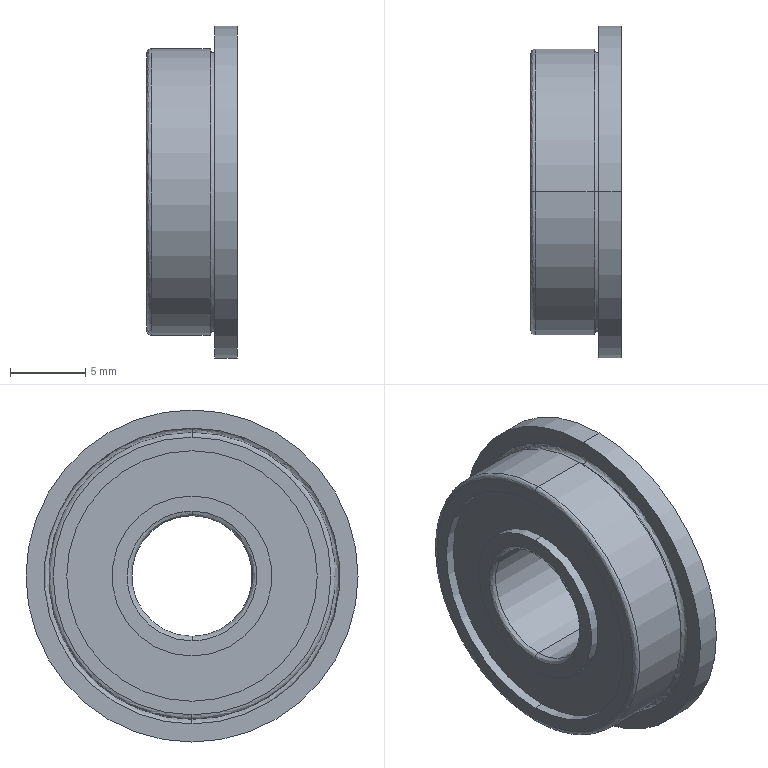Part | SolidWorks | features BaseBody 1 | 1 solid | 31 faces | box 6 x 22 x 22 mm | volume 1366 mm3 | cylinder 14 | spline 11 | plane 6 | commonest cylinder face diameters 10.6 x4 16.6 x4 8 x2 19 x2 22 x2
STEP:
#1=CARTESIAN_POINT('',(4.5,0.,-9.2));
#2=VERTEX_POINT('',#1);
#3=CARTESIAN_POINT('',(4.5,0.,9.2));
#4=VERTEX_POINT('',#3);
#5=CARTESIAN_POINT('',(4.5,0.,0.));
#6=DIRECTION('',(-1.,0.,0.));
#7=DIRECTION('',(0.,0.,1.));
#8=AXIS2_PLACEMENT_3D('',#5,#6,#7);
#9=CIRCLE('',#8,9.2);
#10=EDGE_CURVE('',#2,#4,#9,.T.);
#11=ORIENTED_EDGE('',*,*,#10,.F.);
#12=CARTESIAN_POINT('',(4.5,0.,-9.8));
#13=VERTEX_POINT('',#12);
#14=CARTESIAN_POINT('',(4.5,0.,-9.5));
#15=DIRECTION('',(0.,1.,0.));
#16=DIRECTION('',(0.,0.,1.));
#17=AXIS2_PLACEMENT_3D('',#14,#15,#16);
#18=CIRCLE('',#17,0.3);
#19=EDGE_CURVE('',#2,#13,#18,.T.);
#20=ORIENTED_EDGE('',*,*,#19,.T.);
#21=CARTESIAN_POINT('',(4.5,0.,9.8));
#22=VERTEX_POINT('',#21);
#23=CARTESIAN_POINT('',(4.5,0.,0.));
#24=DIRECTION('',(-1.,0.,0.));
#25=DIRECTION('',(0.,0.,1.));
#26=AXIS2_PLACEMENT_3D('',#23,#24,#25);
#27=CIRCLE('',#26,9.8);
#28=EDGE_CURVE('',#13,#22,#27,.T.);
#29=ORIENTED_EDGE('',*,*,#28,.T.);
#30=CARTESIAN_POINT('',(4.5,0.,9.5));
#31=DIRECTION('',(0.,-1.,0.));
#32=DIRECTION('',(0.,0.,-1.));
#33=AXIS2_PLACEMENT_3D('',#30,#31,#32);
#34=CIRCLE('',#33,0.3);
#35=EDGE_CURVE('',#4,#22,#34,.T.);
#36=ORIENTED_EDGE('',*,*,#35,.F.);
#37=EDGE_LOOP('',(#11,#20,#29,#36));
#38=FACE_OUTER_BOUND('',#37,.T.);
#39=CARTESIAN_POINT('',(4.5,0.,-9.2));
#40=CARTESIAN_POINT('',(4.5,-18.4,-9.2));
#41=CARTESIAN_POINT('',(4.5,-18.4,9.2));
#42=CARTESIAN_POINT('',(4.5,0.,9.2));
#43=CARTESIAN_POINT('',(5.1,0.,-9.2));
#44=CARTESIAN_POINT('',(5.1,-18.4,-9.2));
#45=CARTESIAN_POINT('',(5.1,-18.4,9.2));
#46=CARTESIAN_POINT('',(5.1,0.,9.2));
#47=CARTESIAN_POINT('',(5.1,0.,-9.8));
#48=CARTESIAN_POINT('',(5.1,-19.6,-9.8));
#49=CARTESIAN_POINT('',(5.1,-19.6,9.8));
#50=CARTESIAN_POINT('',(5.1,0.,9.8));
#51=CARTESIAN_POINT('',(4.5,0.,-9.8));
#52=CARTESIAN_POINT('',(4.5,-19.6,-9.8));
#53=CARTESIAN_POINT('',(4.5,-19.6,9.8));
#54=CARTESIAN_POINT('',(4.5,0.,9.8));
#55=(BOUNDED_SURFACE()B_SPLINE_SURFACE(3,3,((#39,#40,#41,#42),(#43,#44,#45,#46),(#47,#48,#49,#50),(#51,#52,#53,#54)),.UNSPECIFIED.,.F.,.F.,.T.)B_SPLINE_SURFACE_WITH_KNOTS((4,4),(4,4),(0.,1.),(0.,1.),.UNSPECIFIED.)GEOMETRIC_REPRESENTATION_ITEM()RATIONAL_B_SPLINE_SURFACE(((1.,0.3333,0.3333,1.),(0.3333,0.1111,0.1111,0.3333),(0.3333,0.1111,0.1111,0.3333),(1.,0.3333,0.3333,1.)))REPRESENTATION_ITEM('')SURFACE());
#56=ADVANCED_FACE('',(#38),#55,.T.);
#57=CARTESIAN_POINT('',(0.,0.,9.2));
#58=VERTEX_POINT('',#57);
#59=CARTESIAN_POINT('',(0.,0.,-9.2));
#60=VERTEX_POINT('',#59);
#61=CARTESIAN_POINT('',(0.,0.,0.));
#62=DIRECTION('',(1.,0.,0.));
#63=DIRECTION('',(0.,0.,1.));
#64=AXIS2_PLACEMENT_3D('',#61,#62,#63);
#65=CIRCLE('',#64,9.2);
#66=EDGE_CURVE('',#58,#60,#65,.T.);
#67=ORIENTED_EDGE('',*,*,#66,.T.);
#68=CARTESIAN_POINT('',(0.3,0.,-9.5));
#69=VERTEX_POINT('',#68);
#70=CARTESIAN_POINT('',(0.3,0.,-9.2));
#71=DIRECTION('',(0.,-1.,0.));
#72=DIRECTION('',(0.,0.,1.));
#73=AXIS2_PLACEMENT_3D('',#70,#71,#72);
#74=CIRCLE('',#73,0.3);
#75=EDGE_CURVE('',#60,#69,#74,.T.);
#76=ORIENTED_EDGE('',*,*,#75,.T.);
#77=CARTESIAN_POINT('',(0.3,0.,9.5));
#78=VERTEX_POINT('',#77);
#79=CARTESIAN_POINT('',(0.3,0.,0.));
#80=DIRECTION('',(1.,0.,0.));
#81=DIRECTION('',(0.,1.,0.));
#82=AXIS2_PLACEMENT_3D('',#79,#80,#81);
#83=CIRCLE('',#82,9.5);
#84=EDGE_CURVE('',#78,#69,#83,.T.);
#85=ORIENTED_EDGE('',*,*,#84,.F.);
#86=CARTESIAN_POINT('',(0.3,0.,9.2));
#87=DIRECTION('',(0.,1.,0.));
#88=DIRECTION('',(0.,0.,-1.));
#89=AXIS2_PLACEMENT_3D('',#86,#87,#88);
#90=CIRCLE('',#89,0.3);
#91=EDGE_CURVE('',#58,#78,#90,.T.);
#92=ORIENTED_EDGE('',*,*,#91,.F.);
#93=EDGE_LOOP('',(#67,#76,#85,#92));
#94=FACE_OUTER_BOUND('',#93,.T.);
#95=CARTESIAN_POINT('',(0.,0.,-9.2));
#96=CARTESIAN_POINT('',(0.,-18.4,-9.2));
#97=CARTESIAN_POINT('',(0.,-18.4,9.2));
#98=CARTESIAN_POINT('',(0.,0.,9.2));
#99=CARTESIAN_POINT('',(0.,0.,-9.376));
#100=CARTESIAN_POINT('',(0.,-18.751,-9.376));
#101=CARTESIAN_POINT('',(0.,-18.751,9.376));
#102=CARTESIAN_POINT('',(0.,0.,9.376));
#103=CARTESIAN_POINT('',(0.1243,0.,-9.5));
#104=CARTESIAN_POINT('',(0.1243,-19.,-9.5));
#105=CARTESIAN_POINT('',(0.1243,-19.,9.5));
#106=CARTESIAN_POINT('',(0.1243,0.,9.5));
#107=CARTESIAN_POINT('',(0.3,0.,-9.5));
#108=CARTESIAN_POINT('',(0.3,-19.,-9.5));
#109=CARTESIAN_POINT('',(0.3,-19.,9.5));
#110=CARTESIAN_POINT('',(0.3,0.,9.5));
#111=(BOUNDED_SURFACE()B_SPLINE_SURFACE(3,3,((#95,#96,#97,#98),(#99,#100,#101,#102),(#103,#104,#105,#106),(#107,#108,#109,#110)),.UNSPECIFIED.,.F.,.F.,.F.)B_SPLINE_SURFACE_WITH_KNOTS((4,4),(4,4),(0.,1.),(0.,1.),.UNSPECIFIED.)GEOMETRIC_REPRESENTATION_ITEM()RATIONAL_B_SPLINE_SURFACE(((1.,0.3333,0.3333,1.),(0.8047,0.2682,0.2682,0.8047),(0.8047,0.2682,0.2682,0.8047),(1.,0.3333,0.3333,1.)))REPRESENTATION_ITEM('')SURFACE());
#112=ADVANCED_FACE('',(#94),#111,.T.);
#113=CARTESIAN_POINT('',(0.3,0.,4.));
#114=VERTEX_POINT('',#113);
#115=CARTESIAN_POINT('',(0.3,0.,-4.));
#116=VERTEX_POINT('',#115);
#117=CARTESIAN_POINT('',(0.3,0.,0.));
#118=DIRECTION('',(1.,0.,0.));
#119=DIRECTION('',(0.,0.,1.));
#120=AXIS2_PLACEMENT_3D('',#117,#118,#119);
#121=CIRCLE('',#120,4.);
#122=EDGE_CURVE('',#114,#116,#121,.T.);
#123=ORIENTED_EDGE('',*,*,#122,.T.);
#124=CARTESIAN_POINT('',(0.,0.,-4.3));
#125=VERTEX_POINT('',#124);
#126=CARTESIAN_POINT('',(0.3,0.,-4.3));
#127=DIRECTION('',(0.,-1.,0.));
#128=DIRECTION('',(0.,0.,1.));
#129=AXIS2_PLACEMENT_3D('',#126,#127,#128);
#130=CIRCLE('',#129,0.3);
#131=EDGE_CURVE('',#116,#125,#130,.T.);
#132=ORIENTED_EDGE('',*,*,#131,.T.);
#133=CARTESIAN_POINT('',(0.,0.,4.3));
#134=VERTEX_POINT('',#133);
#135=CARTESIAN_POINT('',(0.,0.,4.3));
#136=CARTESIAN_POINT('',(0.,-0.2048,4.3));
#137=CARTESIAN_POINT('',(0.,-0.509,4.278));
#138=CARTESIAN_POINT('',(0.,-0.8583,4.216));
#139=CARTESIAN_POINT('',(0.,-1.032,4.175));
#140=CARTESIAN_POINT('',(0.,-1.118,4.152));
#141=CARTESIAN_POINT('',(0.,-1.161,4.14));
#142=CARTESIAN_POINT('',(0.,-1.179,4.135));
#143=CARTESIAN_POINT('',(0.,-1.192,4.132));
#144=CARTESIAN_POINT('',(0.,-1.196,4.13));
#145=CARTESIAN_POINT('',(0.,-1.454,4.055));
#146=CARTESIAN_POINT('',(0.,-1.814,3.914));
#147=CARTESIAN_POINT('',(0.,-2.206,3.695));
#148=CARTESIAN_POINT('',(0.,-2.395,3.572));
#149=CARTESIAN_POINT('',(0.,-2.488,3.507));
#150=CARTESIAN_POINT('',(0.,-2.534,3.474));
#151=CARTESIAN_POINT('',(0.,-2.554,3.459));
#152=CARTESIAN_POINT('',(0.,-2.567,3.45));
#153=CARTESIAN_POINT('',(0.,-2.572,3.446));
#154=CARTESIAN_POINT('',(0.,-2.701,3.35));
#155=CARTESIAN_POINT('',(0.,-2.873,3.205));
#156=CARTESIAN_POINT('',(0.,-3.061,3.021));
#157=CARTESIAN_POINT('',(0.,-3.152,2.926));
#158=CARTESIAN_POINT('',(0.,-3.19,2.884));
#159=CARTESIAN_POINT('',(0.,-3.215,2.856));
#160=CARTESIAN_POINT('',(0.,-3.226,2.843));
#161=CARTESIAN_POINT('',(0.,-3.347,2.704));
#162=CARTESIAN_POINT('',(0.,-3.497,2.511));
#163=CARTESIAN_POINT('',(0.,-3.652,2.272));
#164=CARTESIAN_POINT('',(0.,-3.725,2.149));
#165=CARTESIAN_POINT('',(0.,-3.755,2.095));
#166=CARTESIAN_POINT('',(0.,-3.775,2.06));
#167=CARTESIAN_POINT('',(0.,-3.784,2.043));
#168=CARTESIAN_POINT('',(0.,-3.876,1.87));
#169=CARTESIAN_POINT('',(0.,-3.984,1.635));
#170=CARTESIAN_POINT('',(0.,-4.084,1.35));
#171=CARTESIAN_POINT('',(0.,-4.122,1.226));
#172=CARTESIAN_POINT('',(0.,-4.146,1.143));
#173=CARTESIAN_POINT('',(0.,-4.157,1.102));
#174=CARTESIAN_POINT('',(0.,-4.256,0.7117));
#175=CARTESIAN_POINT('',(0.,-4.3,0.3578));
#176=CARTESIAN_POINT('',(0.,-4.3,-0.1789));
#177=CARTESIAN_POINT('',(0.,-4.284,-0.4454));
#178=CARTESIAN_POINT('',(0.,-4.235,-0.753));
#179=CARTESIAN_POINT('',(0.,-4.208,-0.8842));
#180=CARTESIAN_POINT('',(0.,-4.189,-0.9714));
#181=CARTESIAN_POINT('',(0.,-4.178,-1.016));
#182=CARTESIAN_POINT('',(0.,-4.125,-1.227));
#183=CARTESIAN_POINT('',(0.,-4.046,-1.473));
#184=CARTESIAN_POINT('',(0.,-3.929,-1.752));
#185=CARTESIAN_POINT('',(0.,-3.864,-1.888));
#186=CARTESIAN_POINT('',(0.,-3.834,-1.947));
#187=CARTESIAN_POINT('',(0.,-3.814,-1.985));
#188=CARTESIAN_POINT('',(0.,-3.804,-2.005));
#189=CARTESIAN_POINT('',(0.,-3.717,-2.168));
#190=CARTESIAN_POINT('',(0.,-3.59,-2.377));
#191=CARTESIAN_POINT('',(0.,-3.422,-2.607));
#192=CARTESIAN_POINT('',(0.,-3.332,-2.718));
#193=CARTESIAN_POINT('',(0.,-3.293,-2.765));
#194=CARTESIAN_POINT('',(0.,-3.267,-2.796));
#195=CARTESIAN_POINT('',(0.,-3.252,-2.813));
#196=CARTESIAN_POINT('',(0.,-3.141,-2.941));
#197=CARTESIAN_POINT('',(0.,-2.984,-3.103));
#198=CARTESIAN_POINT('',(0.,-2.787,-3.276));
#199=CARTESIAN_POINT('',(0.,-2.685,-3.359));
#200=CARTESIAN_POINT('',(0.,-2.633,-3.4));
#201=CARTESIAN_POINT('',(0.,-2.61,-3.417));
#202=CARTESIAN_POINT('',(0.,-2.595,-3.429));
#203=CARTESIAN_POINT('',(0.,-2.587,-3.435));
#204=CARTESIAN_POINT('',(0.,-2.372,-3.596));
#205=CARTESIAN_POINT('',(0.,-2.043,-3.799));
#206=CARTESIAN_POINT('',(0.,-1.633,-3.982));
#207=CARTESIAN_POINT('',(0.,-1.421,-4.06));
#208=CARTESIAN_POINT('',(0.,-1.313,-4.095));
#209=CARTESIAN_POINT('',(0.,-1.259,-4.112));
#210=CARTESIAN_POINT('',(0.,-1.235,-4.119));
#211=CARTESIAN_POINT('',(0.,-1.22,-4.123));
#212=CARTESIAN_POINT('',(0.,-1.21,-4.126));
#213=CARTESIAN_POINT('',(0.,-0.8114,-4.243));
#214=CARTESIAN_POINT('',(0.,-0.41,-4.3));
#215=CARTESIAN_POINT('',(0.,0.,-4.3));
#216=B_SPLINE_CURVE_WITH_KNOTS('',3,(#135,#136,#137,#138,#139,#140,#141,#142,#143,#144,#145,#146,#147,#148,#149,#150,#151,#152,#153,#154,#155,#156,#157,#158,#159,#160,#161,#162,#163,#164,#165,#166,#167,#168,#169,#170,#171,#172,#173,#174,#175,#176,#177,#178,#179,#180,#181,#182,#183,#184,#185,#186,#187,#188,#189,#190,#191,#192,#193,#194,#195,#196,#197,#198,#199,#200,#201,#202,#203,#204,#205,#206,#207,#208,#209,#210,#211,#212,#213,#214,#215),.UNSPECIFIED.,.F.,.F.,(4,1,1,1,1,1,2,2,1,1,1,1,1,2,2,1,1,1,2,2,1,1,1,2,2,1,1,2,2,2,1,1,2,2,1,1,1,2,2,1,1,1,2,2,1,1,1,1,2,2,1,1,1,1,1,2,2,4),(0.,0.0625,0.09375,0.1094,0.1172,0.1211,0.123,0.125,0.1875,0.2187,0.2344,0.2422,0.2461,0.248,0.25,0.2812,0.2969,0.3047,0.3086,0.3125,0.3437,0.3594,0.3672,0.3711,0.375,0.4062,0.4219,0.4297,0.4375,0.5,0.5312,0.5469,0.5547,0.5625,0.5937,0.6094,0.6172,0.6211,0.625,0.6562,0.6719,0.6797,0.6836,0.6875,0.7187,0.7344,0.7422,0.7461,0.748,0.75,0.8125,0.8437,0.8594,0.8672,0.8711,0.873,0.875,1.),.UNSPECIFIED.);
#217=EDGE_CURVE('',#134,#125,#216,.T.);
#218=ORIENTED_EDGE('',*,*,#217,.F.);
#219=CARTESIAN_POINT('',(0.3,0.,4.3));
#220=DIRECTION('',(0.,1.,0.));
#221=DIRECTION('',(0.,0.,-1.));
#222=AXIS2_PLACEMENT_3D('',#219,#220,#221);
#223=CIRCLE('',#222,0.3);
#224=EDGE_CURVE('',#114,#134,#223,.T.);
#225=ORIENTED_EDGE('',*,*,#224,.F.);
#226=EDGE_LOOP('',(#123,#132,#218,#225));
#227=FACE_OUTER_BOUND('',#226,.T.);
#228=CARTESIAN_POINT('',(0.3,0.,-4.));
#229=CARTESIAN_POINT('',(0.3,-8.,-4.));
#230=CARTESIAN_POINT('',(0.3,-8.,4.));
#231=CARTESIAN_POINT('',(0.3,0.,4.));
#232=CARTESIAN_POINT('',(0.1243,0.,-4.));
#233=CARTESIAN_POINT('',(0.1243,-8.,-4.));
#234=CARTESIAN_POINT('',(0.1243,-8.,4.));
#235=CARTESIAN_POINT('',(0.1243,0.,4.));
#236=CARTESIAN_POINT('',(0.,0.,-4.124));
#237=CARTESIAN_POINT('',(0.,-8.249,-4.124));
#238=CARTESIAN_POINT('',(0.,-8.249,4.124));
#239=CARTESIAN_POINT('',(0.,0.,4.124));
#240=CARTESIAN_POINT('',(0.,0.,-4.3));
#241=CARTESIAN_POINT('',(0.,-8.6,-4.3));
#242=CARTESIAN_POINT('',(0.,-8.6,4.3));
#243=CARTESIAN_POINT('',(0.,0.,4.3));
#244=(BOUNDED_SURFACE()B_SPLINE_SURFACE(3,3,((#228,#229,#230,#231),(#232,#233,#234,#235),(#236,#237,#238,#239),(#240,#241,#242,#243)),.UNSPECIFIED.,.F.,.F.,.T.)B_SPLINE_SURFACE_WITH_KNOTS((4,4),(4,4),(0.,1.),(0.,1.),.UNSPECIFIED.)GEOMETRIC_REPRESENTATION_ITEM()RATIONAL_B_SPLINE_SURFACE(((1.,0.3333,0.3333,1.),(0.8047,0.2682,0.2682,0.8047),(0.8047,0.2682,0.2682,0.8047),(1.,0.3333,0.3333,1.)))REPRESENTATION_ITEM('')SURFACE());
#245=ADVANCED_FACE('',(#227),#244,.T.);
#246=CARTESIAN_POINT('',(6.,0.,-4.3));
#247=VERTEX_POINT('',#246);
#248=CARTESIAN_POINT('',(6.,0.,4.3));
#249=VERTEX_POINT('',#248);
#250=CARTESIAN_POINT('',(6.,0.,-4.3));
#251=CARTESIAN_POINT('',(6.,-0.2048,-4.3));
#252=CARTESIAN_POINT('',(6.,-0.509,-4.278));
#253=CARTESIAN_POINT('',(6.,-0.8583,-4.216));
#254=CARTESIAN_POINT('',(6.,-1.032,-4.175));
#255=CARTESIAN_POINT('',(6.,-1.118,-4.152));
#256=CARTESIAN_POINT('',(6.,-1.161,-4.14));
#257=CARTESIAN_POINT('',(6.,-1.179,-4.135));
#258=CARTESIAN_POINT('',(6.,-1.192,-4.132));
#259=CARTESIAN_POINT('',(6.,-1.196,-4.13));
#260=CARTESIAN_POINT('',(6.,-1.454,-4.055));
#261=CARTESIAN_POINT('',(6.,-1.814,-3.914));
#262=CARTESIAN_POINT('',(6.,-2.206,-3.695));
#263=CARTESIAN_POINT('',(6.,-2.395,-3.572));
#264=CARTESIAN_POINT('',(6.,-2.488,-3.507));
#265=CARTESIAN_POINT('',(6.,-2.534,-3.474));
#266=CARTESIAN_POINT('',(6.,-2.554,-3.459));
#267=CARTESIAN_POINT('',(6.,-2.567,-3.45));
#268=CARTESIAN_POINT('',(6.,-2.572,-3.446));
#269=CARTESIAN_POINT('',(6.,-2.701,-3.35));
#270=CARTESIAN_POINT('',(6.,-2.873,-3.205));
#271=CARTESIAN_POINT('',(6.,-3.061,-3.021));
#272=CARTESIAN_POINT('',(6.,-3.152,-2.926));
#273=CARTESIAN_POINT('',(6.,-3.19,-2.884));
#274=CARTESIAN_POINT('',(6.,-3.215,-2.856));
#275=CARTESIAN_POINT('',(6.,-3.226,-2.843));
#276=CARTESIAN_POINT('',(6.,-3.347,-2.704));
#277=CARTESIAN_POINT('',(6.,-3.497,-2.511));
#278=CARTESIAN_POINT('',(6.,-3.652,-2.272));
#279=CARTESIAN_POINT('',(6.,-3.725,-2.149));
#280=CARTESIAN_POINT('',(6.,-3.755,-2.095));
#281=CARTESIAN_POINT('',(6.,-3.775,-2.06));
#282=CARTESIAN_POINT('',(6.,-3.784,-2.043));
#283=CARTESIAN_POINT('',(6.,-3.876,-1.87));
#284=CARTESIAN_POINT('',(6.,-3.984,-1.635));
#285=CARTESIAN_POINT('',(6.,-4.084,-1.35));
#286=CARTESIAN_POINT('',(6.,-4.122,-1.226));
#287=CARTESIAN_POINT('',(6.,-4.146,-1.143));
#288=CARTESIAN_POINT('',(6.,-4.157,-1.102));
#289=CARTESIAN_POINT('',(6.,-4.256,-0.7117));
#290=CARTESIAN_POINT('',(6.,-4.3,-0.3578));
#291=CARTESIAN_POINT('',(6.,-4.3,0.1789));
#292=CARTESIAN_POINT('',(6.,-4.284,0.4454));
#293=CARTESIAN_POINT('',(6.,-4.235,0.753));
#294=CARTESIAN_POINT('',(6.,-4.208,0.8842));
#295=CARTESIAN_POINT('',(6.,-4.189,0.9714));
#296=CARTESIAN_POINT('',(6.,-4.178,1.016));
#297=CARTESIAN_POINT('',(6.,-4.125,1.227));
#298=CARTESIAN_POINT('',(6.,-4.046,1.473));
#299=CARTESIAN_POINT('',(6.,-3.929,1.752));
#300=CARTESIAN_POINT('',(6.,-3.864,1.888));
#301=CARTESIAN_POINT('',(6.,-3.834,1.947));
#302=CARTESIAN_POINT('',(6.,-3.814,1.985));
#303=CARTESIAN_POINT('',(6.,-3.804,2.005));
#304=CARTESIAN_POINT('',(6.,-3.717,2.168));
#305=CARTESIAN_POINT('',(6.,-3.59,2.377));
#306=CARTESIAN_POINT('',(6.,-3.422,2.607));
#307=CARTESIAN_POINT('',(6.,-3.332,2.718));
#308=CARTESIAN_POINT('',(6.,-3.293,2.765));
#309=CARTESIAN_POINT('',(6.,-3.267,2.796));
#310=CARTESIAN_POINT('',(6.,-3.252,2.813));
#311=CARTESIAN_POINT('',(6.,-3.141,2.941));
#312=CARTESIAN_POINT('',(6.,-2.984,3.103));
#313=CARTESIAN_POINT('',(6.,-2.787,3.276));
#314=CARTESIAN_POINT('',(6.,-2.685,3.359));
#315=CARTESIAN_POINT('',(6.,-2.633,3.4));
#316=CARTESIAN_POINT('',(6.,-2.61,3.417));
#317=CARTESIAN_POINT('',(6.,-2.595,3.429));
#318=CARTESIAN_POINT('',(6.,-2.587,3.435));
#319=CARTESIAN_POINT('',(6.,-2.372,3.596));
#320=CARTESIAN_POINT('',(6.,-2.043,3.799));
#321=CARTESIAN_POINT('',(6.,-1.633,3.982));
#322=CARTESIAN_POINT('',(6.,-1.421,4.06));
#323=CARTESIAN_POINT('',(6.,-1.313,4.095));
#324=CARTESIAN_POINT('',(6.,-1.259,4.112));
#325=CARTESIAN_POINT('',(6.,-1.235,4.119));
#326=CARTESIAN_POINT('',(6.,-1.22,4.123));
#327=CARTESIAN_POINT('',(6.,-1.21,4.126));
#328=CARTESIAN_POINT('',(6.,-0.8114,4.243));
#329=CARTESIAN_POINT('',(6.,-0.41,4.3));
#330=CARTESIAN_POINT('',(6.,0.,4.3));
#331=B_SPLINE_CURVE_WITH_KNOTS('',3,(#250,#251,#252,#253,#254,#255,#256,#257,#258,#259,#260,#261,#262,#263,#264,#265,#266,#267,#268,#269,#270,#271,#272,#273,#274,#275,#276,#277,#278,#279,#280,#281,#282,#283,#284,#285,#286,#287,#288,#289,#290,#291,#292,#293,#294,#295,#296,#297,#298,#299,#300,#301,#302,#303,#304,#305,#306,#307,#308,#309,#310,#311,#312,#313,#314,#315,#316,#317,#318,#319,#320,#321,#322,#323,#324,#325,#326,#327,#328,#329,#330),.UNSPECIFIED.,.F.,.F.,(4,1,1,1,1,1,2,2,1,1,1,1,1,2,2,1,1,1,2,2,1,1,1,2,2,1,1,2,2,2,1,1,2,2,1,1,1,2,2,1,1,1,2,2,1,1,1,1,2,2,1,1,1,1,1,2,2,4),(0.,0.0625,0.09375,0.1094,0.1172,0.1211,0.123,0.125,0.1875,0.2187,0.2344,0.2422,0.2461,0.248,0.25,0.2812,0.2969,0.3047,0.3086,0.3125,0.3437,0.3594,0.3672,0.3711,0.375,0.4062,0.4219,0.4297,0.4375,0.5,0.5312,0.5469,0.5547,0.5625,0.5937,0.6094,0.6172,0.6211,0.625,0.6562,0.6719,0.6797,0.6836,0.6875,0.7187,0.7344,0.7422,0.7461,0.748,0.75,0.8125,0.8437,0.8594,0.8672,0.8711,0.873,0.875,1.),.UNSPECIFIED.);
#332=EDGE_CURVE('',#247,#249,#331,.T.);
#333=ORIENTED_EDGE('',*,*,#332,.F.);
#334=CARTESIAN_POINT('',(5.7,0.,-4.));
#335=VERTEX_POINT('',#334);
#336=CARTESIAN_POINT('',(5.7,0.,-4.3));
#337=DIRECTION('',(0.,-1.,0.));
#338=DIRECTION('',(0.,0.,1.));
#339=AXIS2_PLACEMENT_3D('',#336,#337,#338);
#340=CIRCLE('',#339,0.3);
#341=EDGE_CURVE('',#247,#335,#340,.T.);
#342=ORIENTED_EDGE('',*,*,#341,.T.);
#343=CARTESIAN_POINT('',(5.7,0.,4.));
#344=VERTEX_POINT('',#343);
#345=CARTESIAN_POINT('',(5.7,0.,0.));
#346=DIRECTION('',(1.,0.,0.));
#347=DIRECTION('',(0.,1.,0.));
#348=AXIS2_PLACEMENT_3D('',#345,#346,#347);
#349=CIRCLE('',#348,4.);
#350=EDGE_CURVE('',#344,#335,#349,.T.);
#351=ORIENTED_EDGE('',*,*,#350,.F.);
#352=CARTESIAN_POINT('',(5.7,0.,4.3));
#353=DIRECTION('',(0.,1.,0.));
#354=DIRECTION('',(0.,0.,-1.));
#355=AXIS2_PLACEMENT_3D('',#352,#353,#354);
#356=CIRCLE('',#355,0.3);
#357=EDGE_CURVE('',#249,#344,#356,.T.);
#358=ORIENTED_EDGE('',*,*,#357,.F.);
#359=EDGE_LOOP('',(#333,#342,#351,#358));
#360=FACE_OUTER_BOUND('',#359,.T.);
#361=CARTESIAN_POINT('',(6.,0.,-4.3));
#362=CARTESIAN_POINT('',(6.,-8.6,-4.3));
#363=CARTESIAN_POINT('',(6.,-8.6,4.3));
#364=CARTESIAN_POINT('',(6.,0.,4.3));
#365=CARTESIAN_POINT('',(6.,0.,-4.124));
#366=CARTESIAN_POINT('',(6.,-8.249,-4.124));
#367=CARTESIAN_POINT('',(6.,-8.249,4.124));
#368=CARTESIAN_POINT('',(6.,0.,4.124));
#369=CARTESIAN_POINT('',(5.876,0.,-4.));
#370=CARTESIAN_POINT('',(5.876,-8.,-4.));
#371=CARTESIAN_POINT('',(5.876,-8.,4.));
#372=CARTESIAN_POINT('',(5.876,0.,4.));
#373=CARTESIAN_POINT('',(5.7,0.,-4.));
#374=CARTESIAN_POINT('',(5.7,-8.,-4.));
#375=CARTESIAN_POINT('',(5.7,-8.,4.));
#376=CARTESIAN_POINT('',(5.7,0.,4.));
#377=(BOUNDED_SURFACE()B_SPLINE_SURFACE(3,3,((#361,#362,#363,#364),(#365,#366,#367,#368),(#369,#370,#371,#372),(#373,#374,#375,#376)),.UNSPECIFIED.,.F.,.F.,.F.)B_SPLINE_SURFACE_WITH_KNOTS((4,4),(4,4),(0.,1.),(0.,1.),.UNSPECIFIED.)GEOMETRIC_REPRESENTATION_ITEM()RATIONAL_B_SPLINE_SURFACE(((1.,0.3333,0.3333,1.),(0.8047,0.2682,0.2682,0.8047),(0.8047,0.2682,0.2682,0.8047),(1.,0.3333,0.3333,1.)))REPRESENTATION_ITEM('')SURFACE());
#378=ADVANCED_FACE('',(#360),#377,.T.);
#379=CARTESIAN_POINT('',(4.2,0.,9.5));
#380=VERTEX_POINT('',#379);
#381=CARTESIAN_POINT('',(4.2,0.,-9.5));
#382=VERTEX_POINT('',#381);
#383=CARTESIAN_POINT('',(4.2,0.,0.));
#384=DIRECTION('',(1.,0.,0.));
#385=DIRECTION('',(0.,0.,1.));
#386=AXIS2_PLACEMENT_3D('',#383,#384,#385);
#387=CIRCLE('',#386,9.5);
#388=EDGE_CURVE('',#380,#382,#387,.T.);
#389=ORIENTED_EDGE('',*,*,#388,.T.);
#390=CARTESIAN_POINT('',(4.5,0.,-9.5));
#391=DIRECTION('',(0.,1.,0.));
#392=DIRECTION('',(0.,0.,1.));
#393=AXIS2_PLACEMENT_3D('',#390,#391,#392);
#394=CIRCLE('',#393,0.3);
#395=EDGE_CURVE('',#382,#2,#394,.T.);
#396=ORIENTED_EDGE('',*,*,#395,.T.);
#397=ORIENTED_EDGE('',*,*,#10,.T.);
#398=CARTESIAN_POINT('',(4.5,0.,9.5));
#399=DIRECTION('',(0.,-1.,0.));
#400=DIRECTION('',(0.,0.,-1.));
#401=AXIS2_PLACEMENT_3D('',#398,#399,#400);
#402=CIRCLE('',#401,0.3);
#403=EDGE_CURVE('',#380,#4,#402,.T.);
#404=ORIENTED_EDGE('',*,*,#403,.F.);
#405=EDGE_LOOP('',(#389,#396,#397,#404));
#406=FACE_OUTER_BOUND('',#405,.T.);
#407=CARTESIAN_POINT('',(4.2,0.,-9.5));
#408=CARTESIAN_POINT('',(4.2,-19.,-9.5));
#409=CARTESIAN_POINT('',(4.2,-19.,9.5));
#410=CARTESIAN_POINT('',(4.2,0.,9.5));
#411=CARTESIAN_POINT('',(4.2,0.,-9.324));
#412=CARTESIAN_POINT('',(4.2,-18.649,-9.324));
#413=CARTESIAN_POINT('',(4.2,-18.649,9.324));
#414=CARTESIAN_POINT('',(4.2,0.,9.324));
#415=CARTESIAN_POINT('',(4.324,0.,-9.2));
#416=CARTESIAN_POINT('',(4.324,-18.4,-9.2));
#417=CARTESIAN_POINT('',(4.324,-18.4,9.2));
#418=CARTESIAN_POINT('',(4.324,0.,9.2));
#419=CARTESIAN_POINT('',(4.5,0.,-9.2));
#420=CARTESIAN_POINT('',(4.5,-18.4,-9.2));
#421=CARTESIAN_POINT('',(4.5,-18.4,9.2));
#422=CARTESIAN_POINT('',(4.5,0.,9.2));
#423=(BOUNDED_SURFACE()B_SPLINE_SURFACE(3,3,((#407,#408,#409,#410),(#411,#412,#413,#414),(#415,#416,#417,#418),(#419,#420,#421,#422)),.UNSPECIFIED.,.F.,.F.,.F.)B_SPLINE_SURFACE_WITH_KNOTS((4,4),(4,4),(0.,1.),(0.,1.),.UNSPECIFIED.)GEOMETRIC_REPRESENTATION_ITEM()RATIONAL_B_SPLINE_SURFACE(((1.,0.3333,0.3333,1.),(0.8047,0.2682,0.2682,0.8047),(0.8047,0.2682,0.2682,0.8047),(1.,0.3333,0.3333,1.)))REPRESENTATION_ITEM('')SURFACE());
#424=ADVANCED_FACE('',(#406),#423,.T.);
#425=ORIENTED_EDGE('',*,*,#395,.F.);
#426=CARTESIAN_POINT('',(4.2,0.,0.));
#427=DIRECTION('',(1.,0.,0.));
#428=DIRECTION('',(0.,0.,1.));
#429=AXIS2_PLACEMENT_3D('',#426,#427,#428);
#430=CIRCLE('',#429,9.5);
#431=EDGE_CURVE('',#382,#380,#430,.T.);
#432=ORIENTED_EDGE('',*,*,#431,.T.);
#433=ORIENTED_EDGE('',*,*,#403,.T.);
#434=CARTESIAN_POINT('',(4.5,0.,0.));
#435=DIRECTION('',(-1.,0.,0.));
#436=DIRECTION('',(0.,0.,1.));
#437=AXIS2_PLACEMENT_3D('',#434,#435,#436);
#438=CIRCLE('',#437,9.2);
#439=EDGE_CURVE('',#4,#2,#438,.T.);
#440=ORIENTED_EDGE('',*,*,#439,.T.);
#441=EDGE_LOOP('',(#425,#432,#433,#440));
#442=FACE_OUTER_BOUND('',#441,.T.);
#443=CARTESIAN_POINT('',(4.2,0.,9.5));
#444=CARTESIAN_POINT('',(4.2,19.,9.5));
#445=CARTESIAN_POINT('',(4.2,19.,-9.5));
#446=CARTESIAN_POINT('',(4.2,0.,-9.5));
#447=CARTESIAN_POINT('',(4.2,0.,9.324));
#448=CARTESIAN_POINT('',(4.2,18.649,9.324));
#449=CARTESIAN_POINT('',(4.2,18.649,-9.324));
#450=CARTESIAN_POINT('',(4.2,0.,-9.324));
#451=CARTESIAN_POINT('',(4.324,0.,9.2));
#452=CARTESIAN_POINT('',(4.324,18.4,9.2));
#453=CARTESIAN_POINT('',(4.324,18.4,-9.2));
#454=CARTESIAN_POINT('',(4.324,0.,-9.2));
#455=CARTESIAN_POINT('',(4.5,0.,9.2));
#456=CARTESIAN_POINT('',(4.5,18.4,9.2));
#457=CARTESIAN_POINT('',(4.5,18.4,-9.2));
#458=CARTESIAN_POINT('',(4.5,0.,-9.2));
#459=(BOUNDED_SURFACE()B_SPLINE_SURFACE(3,3,((#443,#444,#445,#446),(#447,#448,#449,#450),(#451,#452,#453,#454),(#455,#456,#457,#458)),.UNSPECIFIED.,.F.,.F.,.T.)B_SPLINE_SURFACE_WITH_KNOTS((4,4),(4,4),(0.,1.),(0.,1.),.UNSPECIFIED.)GEOMETRIC_REPRESENTATION_ITEM()RATIONAL_B_SPLINE_SURFACE(((1.,0.3333,0.3333,1.),(0.8047,0.2682,0.2682,0.8047),(0.8047,0.2682,0.2682,0.8047),(1.,0.3333,0.3333,1.)))REPRESENTATION_ITEM('')SURFACE());
#460=ADVANCED_FACE('',(#442),#459,.T.);
#461=ORIENTED_EDGE('',*,*,#431,.F.);
#462=CARTESIAN_POINT('',(0.3,0.,-9.5));
#463=DIRECTION('',(-1.,0.,0.));
#464=VECTOR('',#463,1000.);
#465=LINE('',#462,#464);
#466=EDGE_CURVE('',#382,#69,#465,.T.);
#467=ORIENTED_EDGE('',*,*,#466,.T.);
#468=CARTESIAN_POINT('',(0.3,0.,0.));
#469=DIRECTION('',(1.,0.,0.));
#470=DIRECTION('',(0.,1.,0.));
#471=AXIS2_PLACEMENT_3D('',#468,#469,#470);
#472=CIRCLE('',#471,9.5);
#473=EDGE_CURVE('',#69,#78,#472,.T.);
#474=ORIENTED_EDGE('',*,*,#473,.T.);
#475=CARTESIAN_POINT('',(0.3,0.,9.5));
#476=DIRECTION('',(-1.,0.,0.));
#477=VECTOR('',#476,1000.);
#478=LINE('',#475,#477);
#479=EDGE_CURVE('',#380,#78,#478,.T.);
#480=ORIENTED_EDGE('',*,*,#479,.F.);
#481=EDGE_LOOP('',(#461,#467,#474,#480));
#482=FACE_OUTER_BOUND('',#481,.T.);
#483=CARTESIAN_POINT('',(0.3,0.,0.));
#484=DIRECTION('',(-1.,0.,0.));
#485=DIRECTION('',(0.,0.,1.));
#486=AXIS2_PLACEMENT_3D('',#483,#484,#485);
#487=CYLINDRICAL_SURFACE('',#486,9.5);
#488=ADVANCED_FACE('',(#482),#487,.T.);
#489=CARTESIAN_POINT('',(6.,0.,11.));
#490=VERTEX_POINT('',#489);
#491=CARTESIAN_POINT('',(6.,0.,-11.));
#492=VERTEX_POINT('',#491);
#493=CARTESIAN_POINT('',(6.,0.,0.));
#494=DIRECTION('',(-1.,0.,0.));
#495=DIRECTION('',(0.,0.,1.));
#496=AXIS2_PLACEMENT_3D('',#493,#494,#495);
#497=CIRCLE('',#496,11.);
#498=EDGE_CURVE('',#490,#492,#497,.T.);
#499=ORIENTED_EDGE('',*,*,#498,.T.);
#500=CARTESIAN_POINT('',(4.5,0.,-11.));
#501=VERTEX_POINT('',#500);
#502=CARTESIAN_POINT('',(4.5,0.,-11.));
#503=DIRECTION('',(-1.,0.,0.));
#504=VECTOR('',#503,1000.);
#505=LINE('',#502,#504);
#506=EDGE_CURVE('',#492,#501,#505,.T.);
#507=ORIENTED_EDGE('',*,*,#506,.T.);
#508=CARTESIAN_POINT('',(4.5,0.,11.));
#509=VERTEX_POINT('',#508);
#510=CARTESIAN_POINT('',(4.5,0.,0.));
#511=DIRECTION('',(-1.,0.,0.));
#512=DIRECTION('',(0.,0.,1.));
#513=AXIS2_PLACEMENT_3D('',#510,#511,#512);
#514=CIRCLE('',#513,11.);
#515=EDGE_CURVE('',#509,#501,#514,.T.);
#516=ORIENTED_EDGE('',*,*,#515,.F.);
#517=CARTESIAN_POINT('',(4.5,0.,11.));
#518=DIRECTION('',(-1.,0.,0.));
#519=VECTOR('',#518,1000.);
#520=LINE('',#517,#519);
#521=EDGE_CURVE('',#490,#509,#520,.T.);
#522=ORIENTED_EDGE('',*,*,#521,.F.);
#523=EDGE_LOOP('',(#499,#507,#516,#522));
#524=FACE_OUTER_BOUND('',#523,.T.);
#525=CARTESIAN_POINT('',(4.5,0.,0.));
#526=DIRECTION('',(-1.,0.,0.));
#527=DIRECTION('',(0.,0.,1.));
#528=AXIS2_PLACEMENT_3D('',#525,#526,#527);
#529=CYLINDRICAL_SURFACE('',#528,11.);
#530=ADVANCED_FACE('',(#524),#529,.T.);
#531=CARTESIAN_POINT('',(0.64,0.,8.3));
#532=VERTEX_POINT('',#531);
#533=CARTESIAN_POINT('',(0.64,0.,-8.3));
#534=VERTEX_POINT('',#533);
#535=CARTESIAN_POINT('',(0.64,0.,0.));
#536=DIRECTION('',(1.,0.,0.));
#537=DIRECTION('',(0.,0.,1.));
#538=AXIS2_PLACEMENT_3D('',#535,#536,#537);
#539=CIRCLE('',#538,8.3);
#540=EDGE_CURVE('',#532,#534,#539,.T.);
#541=ORIENTED_EDGE('',*,*,#540,.T.);
#542=CARTESIAN_POINT('',(0.,0.,-8.3));
#543=VERTEX_POINT('',#542);
#544=CARTESIAN_POINT('',(0.64,0.,-8.3));
#545=DIRECTION('',(-1.,0.,0.));
#546=VECTOR('',#545,1000.);
#547=LINE('',#544,#546);
#548=EDGE_CURVE('',#534,#543,#547,.T.);
#549=ORIENTED_EDGE('',*,*,#548,.T.);
#550=CARTESIAN_POINT('',(0.,0.,8.3));
#551=VERTEX_POINT('',#550);
#552=CARTESIAN_POINT('',(0.,0.,0.));
#553=DIRECTION('',(1.,0.,0.));
#554=DIRECTION('',(0.,0.,1.));
#555=AXIS2_PLACEMENT_3D('',#552,#553,#554);
#556=CIRCLE('',#555,8.3);
#557=EDGE_CURVE('',#551,#543,#556,.T.);
#558=ORIENTED_EDGE('',*,*,#557,.F.);
#559=CARTESIAN_POINT('',(0.64,0.,8.3));
#560=DIRECTION('',(-1.,0.,0.));
#561=VECTOR('',#560,1000.);
#562=LINE('',#559,#561);
#563=EDGE_CURVE('',#532,#551,#562,.T.);
#564=ORIENTED_EDGE('',*,*,#563,.F.);
#565=EDGE_LOOP('',(#541,#549,#558,#564));
#566=FACE_OUTER_BOUND('',#565,.T.);
#567=CARTESIAN_POINT('',(0.64,0.,0.));
#568=DIRECTION('',(-1.,0.,0.));
#569=DIRECTION('',(0.,0.,1.));
#570=AXIS2_PLACEMENT_3D('',#567,#568,#569);
#571=CYLINDRICAL_SURFACE('',#570,8.3);
#572=ADVANCED_FACE('',(#566),#571,.F.);
#573=CARTESIAN_POINT('',(6.,0.,-8.3));
#574=VERTEX_POINT('',#573);
#575=CARTESIAN_POINT('',(6.,0.,8.3));
#576=VERTEX_POINT('',#575);
#577=CARTESIAN_POINT('',(6.,0.,0.));
#578=DIRECTION('',(-1.,0.,0.));
#579=DIRECTION('',(0.,0.,1.));
#580=AXIS2_PLACEMENT_3D('',#577,#578,#579);
#581=CIRCLE('',#580,8.3);
#582=EDGE_CURVE('',#574,#576,#581,.T.);
#583=ORIENTED_EDGE('',*,*,#582,.F.);
#584=CARTESIAN_POINT('',(5.36,0.,-8.3));
#585=VERTEX_POINT('',#584);
#586=CARTESIAN_POINT('',(6.,0.,-8.3));
#587=DIRECTION('',(-1.,0.,0.));
#588=VECTOR('',#587,1000.);
#589=LINE('',#586,#588);
#590=EDGE_CURVE('',#574,#585,#589,.T.);
#591=ORIENTED_EDGE('',*,*,#590,.T.);
#592=CARTESIAN_POINT('',(5.36,0.,8.3));
#593=VERTEX_POINT('',#592);
#594=CARTESIAN_POINT('',(5.36,0.,0.));
#595=DIRECTION('',(-1.,0.,0.));
#596=DIRECTION('',(0.,0.,1.));
#597=AXIS2_PLACEMENT_3D('',#594,#595,#596);
#598=CIRCLE('',#597,8.3);
#599=EDGE_CURVE('',#585,#593,#598,.T.);
#600=ORIENTED_EDGE('',*,*,#599,.T.);
#601=CARTESIAN_POINT('',(6.,0.,8.3));
#602=DIRECTION('',(-1.,0.,0.));
#603=VECTOR('',#602,1000.);
#604=LINE('',#601,#603);
#605=EDGE_CURVE('',#576,#593,#604,.T.);
#606=ORIENTED_EDGE('',*,*,#605,.F.);
#607=EDGE_LOOP('',(#583,#591,#600,#606));
#608=FACE_OUTER_BOUND('',#607,.T.);
#609=CARTESIAN_POINT('',(6.,0.,0.));
#610=DIRECTION('',(-1.,0.,0.));
#611=DIRECTION('',(0.,0.,1.));
#612=AXIS2_PLACEMENT_3D('',#609,#610,#611);
#613=CYLINDRICAL_SURFACE('',#612,8.3);
#614=ADVANCED_FACE('',(#608),#613,.F.);
#615=CARTESIAN_POINT('',(0.64,0.,-5.3));
#616=VERTEX_POINT('',#615);
#617=CARTESIAN_POINT('',(0.64,0.,5.3));
#618=VERTEX_POINT('',#617);
#619=CARTESIAN_POINT('',(0.64,0.,0.));
#620=DIRECTION('',(1.,0.,0.));
#621=DIRECTION('',(0.,0.,1.));
#622=AXIS2_PLACEMENT_3D('',#619,#620,#621);
#623=CIRCLE('',#622,5.3);
#624=EDGE_CURVE('',#616,#618,#623,.T.);
#625=ORIENTED_EDGE('',*,*,#624,.F.);
#626=CARTESIAN_POINT('',(0.,0.,-5.3));
#627=VERTEX_POINT('',#626);
#628=CARTESIAN_POINT('',(0.,0.,-5.3));
#629=DIRECTION('',(-1.,0.,0.));
#630=VECTOR('',#629,1000.);
#631=LINE('',#628,#630);
#632=EDGE_CURVE('',#616,#627,#631,.T.);
#633=ORIENTED_EDGE('',*,*,#632,.T.);
#634=CARTESIAN_POINT('',(0.,0.,5.3));
#635=VERTEX_POINT('',#634);
#636=CARTESIAN_POINT('',(0.,0.,0.));
#637=DIRECTION('',(1.,0.,0.));
#638=DIRECTION('',(0.,0.,1.));
#639=AXIS2_PLACEMENT_3D('',#636,#637,#638);
#640=CIRCLE('',#639,5.3);
#641=EDGE_CURVE('',#627,#635,#640,.T.);
#642=ORIENTED_EDGE('',*,*,#641,.T.);
#643=CARTESIAN_POINT('',(0.,0.,5.3));
#644=DIRECTION('',(-1.,0.,0.));
#645=VECTOR('',#644,1000.);
#646=LINE('',#643,#645);
#647=EDGE_CURVE('',#618,#635,#646,.T.);
#648=ORIENTED_EDGE('',*,*,#647,.F.);
#649=EDGE_LOOP('',(#625,#633,#642,#648));
#650=FACE_OUTER_BOUND('',#649,.T.);
#651=CARTESIAN_POINT('',(0.,0.,0.));
#652=DIRECTION('',(-1.,0.,0.));
#653=DIRECTION('',(0.,0.,1.));
#654=AXIS2_PLACEMENT_3D('',#651,#652,#653);
#655=CYLINDRICAL_SURFACE('',#654,5.3);
#656=ADVANCED_FACE('',(#650),#655,.T.);
#657=CARTESIAN_POINT('',(6.,0.,5.3));
#658=VERTEX_POINT('',#657);
#659=CARTESIAN_POINT('',(6.,0.,-5.3));
#660=VERTEX_POINT('',#659);
#661=CARTESIAN_POINT('',(6.,0.,0.));
#662=DIRECTION('',(-1.,0.,0.));
#663=DIRECTION('',(0.,0.,1.));
#664=AXIS2_PLACEMENT_3D('',#661,#662,#663);
#665=CIRCLE('',#664,5.3);
#666=EDGE_CURVE('',#658,#660,#665,.T.);
#667=ORIENTED_EDGE('',*,*,#666,.T.);
#668=CARTESIAN_POINT('',(5.36,0.,-5.3));
#669=VERTEX_POINT('',#668);
#670=CARTESIAN_POINT('',(5.36,0.,-5.3));
#671=DIRECTION('',(-1.,0.,0.));
#672=VECTOR('',#671,1000.);
#673=LINE('',#670,#672);
#674=EDGE_CURVE('',#660,#669,#673,.T.);
#675=ORIENTED_EDGE('',*,*,#674,.T.);
#676=CARTESIAN_POINT('',(5.36,0.,5.3));
#677=VERTEX_POINT('',#676);
#678=CARTESIAN_POINT('',(5.36,0.,0.));
#679=DIRECTION('',(-1.,0.,0.));
#680=DIRECTION('',(0.,0.,1.));
#681=AXIS2_PLACEMENT_3D('',#678,#679,#680);
#682=CIRCLE('',#681,5.3);
#683=EDGE_CURVE('',#677,#669,#682,.T.);
#684=ORIENTED_EDGE('',*,*,#683,.F.);
#685=CARTESIAN_POINT('',(5.36,0.,5.3));
#686=DIRECTION('',(-1.,0.,0.));
#687=VECTOR('',#686,1000.);
#688=LINE('',#685,#687);
#689=EDGE_CURVE('',#658,#677,#688,.T.);
#690=ORIENTED_EDGE('',*,*,#689,.F.);
#691=EDGE_LOOP('',(#667,#675,#684,#690));
#692=FACE_OUTER_BOUND('',#691,.T.);
#693=CARTESIAN_POINT('',(5.36,0.,0.));
#694=DIRECTION('',(-1.,0.,0.));
#695=DIRECTION('',(0.,0.,1.));
#696=AXIS2_PLACEMENT_3D('',#693,#694,#695);
#697=CYLINDRICAL_SURFACE('',#696,5.3);
#698=ADVANCED_FACE('',(#692),#697,.T.);
#699=ORIENTED_EDGE('',*,*,#350,.T.);
#700=CARTESIAN_POINT('',(5.7,0.,-4.));
#701=DIRECTION('',(-1.,0.,0.));
#702=VECTOR('',#701,1000.);
#703=LINE('',#700,#702);
#704=EDGE_CURVE('',#335,#116,#703,.T.);
#705=ORIENTED_EDGE('',*,*,#704,.T.);
#706=ORIENTED_EDGE('',*,*,#122,.F.);
#707=CARTESIAN_POINT('',(5.7,0.,4.));
#708=DIRECTION('',(-1.,0.,0.));
#709=VECTOR('',#708,1000.);
#710=LINE('',#707,#709);
#711=EDGE_CURVE('',#344,#114,#710,.T.);
#712=ORIENTED_EDGE('',*,*,#711,.F.);
#713=EDGE_LOOP('',(#699,#705,#706,#712));
#714=FACE_OUTER_BOUND('',#713,.T.);
#715=CARTESIAN_POINT('',(5.7,0.,0.));
#716=DIRECTION('',(-1.,0.,0.));
#717=DIRECTION('',(0.,0.,1.));
#718=AXIS2_PLACEMENT_3D('',#715,#716,#717);
#719=CYLINDRICAL_SURFACE('',#718,4.);
#720=ADVANCED_FACE('',(#714),#719,.F.);
#721=ORIENTED_EDGE('',*,*,#19,.F.);
#722=ORIENTED_EDGE('',*,*,#439,.F.);
#723=ORIENTED_EDGE('',*,*,#35,.T.);
#724=CARTESIAN_POINT('',(4.5,0.,0.));
#725=DIRECTION('',(-1.,0.,0.));
#726=DIRECTION('',(0.,0.,1.));
#727=AXIS2_PLACEMENT_3D('',#724,#725,#726);
#728=CIRCLE('',#727,9.8);
#729=EDGE_CURVE('',#22,#13,#728,.T.);
#730=ORIENTED_EDGE('',*,*,#729,.T.);
#731=EDGE_LOOP('',(#721,#722,#723,#730));
#732=FACE_OUTER_BOUND('',#731,.T.);
#733=CARTESIAN_POINT('',(4.5,0.,9.2));
#734=CARTESIAN_POINT('',(4.5,18.4,9.2));
#735=CARTESIAN_POINT('',(4.5,18.4,-9.2));
#736=CARTESIAN_POINT('',(4.5,0.,-9.2));
#737=CARTESIAN_POINT('',(5.1,0.,9.2));
#738=CARTESIAN_POINT('',(5.1,18.4,9.2));
#739=CARTESIAN_POINT('',(5.1,18.4,-9.2));
#740=CARTESIAN_POINT('',(5.1,0.,-9.2));
#741=CARTESIAN_POINT('',(5.1,0.,9.8));
#742=CARTESIAN_POINT('',(5.1,19.6,9.8));
#743=CARTESIAN_POINT('',(5.1,19.6,-9.8));
#744=CARTESIAN_POINT('',(5.1,0.,-9.8));
#745=CARTESIAN_POINT('',(4.5,0.,9.8));
#746=CARTESIAN_POINT('',(4.5,19.6,9.8));
#747=CARTESIAN_POINT('',(4.5,19.6,-9.8));
#748=CARTESIAN_POINT('',(4.5,0.,-9.8));
#749=(BOUNDED_SURFACE()B_SPLINE_SURFACE(3,3,((#733,#734,#735,#736),(#737,#738,#739,#740),(#741,#742,#743,#744),(#745,#746,#747,#748)),.UNSPECIFIED.,.F.,.F.,.F.)B_SPLINE_SURFACE_WITH_KNOTS((4,4),(4,4),(0.,1.),(0.,1.),.UNSPECIFIED.)GEOMETRIC_REPRESENTATION_ITEM()RATIONAL_B_SPLINE_SURFACE(((1.,0.3333,0.3333,1.),(0.3333,0.1111,0.1111,0.3333),(0.3333,0.1111,0.1111,0.3333),(1.,0.3333,0.3333,1.)))REPRESENTATION_ITEM('')SURFACE());
#750=ADVANCED_FACE('',(#732),#749,.T.);
#751=ORIENTED_EDGE('',*,*,#466,.F.);
#752=ORIENTED_EDGE('',*,*,#388,.F.);
#753=ORIENTED_EDGE('',*,*,#479,.T.);
#754=ORIENTED_EDGE('',*,*,#84,.T.);
#755=EDGE_LOOP('',(#751,#752,#753,#754));
#756=FACE_OUTER_BOUND('',#755,.T.);
#757=CARTESIAN_POINT('',(0.3,0.,0.));
#758=DIRECTION('',(-1.,0.,0.));
#759=DIRECTION('',(0.,0.,1.));
#760=AXIS2_PLACEMENT_3D('',#757,#758,#759);
#761=CYLINDRICAL_SURFACE('',#760,9.5);
#762=ADVANCED_FACE('',(#756),#761,.T.);
#763=ORIENTED_EDGE('',*,*,#75,.F.);
#764=CARTESIAN_POINT('',(0.,0.,0.));
#765=DIRECTION('',(1.,0.,0.));
#766=DIRECTION('',(0.,0.,1.));
#767=AXIS2_PLACEMENT_3D('',#764,#765,#766);
#768=CIRCLE('',#767,9.2);
#769=EDGE_CURVE('',#60,#58,#768,.T.);
#770=ORIENTED_EDGE('',*,*,#769,.T.);
#771=ORIENTED_EDGE('',*,*,#91,.T.);
#772=ORIENTED_EDGE('',*,*,#473,.F.);
#773=EDGE_LOOP('',(#763,#770,#771,#772));
#774=FACE_OUTER_BOUND('',#773,.T.);
#775=CARTESIAN_POINT('',(0.,0.,9.2));
#776=CARTESIAN_POINT('',(0.,18.4,9.2));
#777=CARTESIAN_POINT('',(0.,18.4,-9.2));
#778=CARTESIAN_POINT('',(0.,0.,-9.2));
#779=CARTESIAN_POINT('',(0.,0.,9.376));
#780=CARTESIAN_POINT('',(0.,18.751,9.376));
#781=CARTESIAN_POINT('',(0.,18.751,-9.376));
#782=CARTESIAN_POINT('',(0.,0.,-9.376));
#783=CARTESIAN_POINT('',(0.1243,0.,9.5));
#784=CARTESIAN_POINT('',(0.1243,19.,9.5));
#785=CARTESIAN_POINT('',(0.1243,19.,-9.5));
#786=CARTESIAN_POINT('',(0.1243,0.,-9.5));
#787=CARTESIAN_POINT('',(0.3,0.,9.5));
#788=CARTESIAN_POINT('',(0.3,19.,9.5));
#789=CARTESIAN_POINT('',(0.3,19.,-9.5));
#790=CARTESIAN_POINT('',(0.3,0.,-9.5));
#791=(BOUNDED_SURFACE()B_SPLINE_SURFACE(3,3,((#775,#776,#777,#778),(#779,#780,#781,#782),(#783,#784,#785,#786),(#787,#788,#789,#790)),.UNSPECIFIED.,.F.,.F.,.F.)B_SPLINE_SURFACE_WITH_KNOTS((4,4),(4,4),(0.,1.),(0.,1.),.UNSPECIFIED.)GEOMETRIC_REPRESENTATION_ITEM()RATIONAL_B_SPLINE_SURFACE(((1.,0.3333,0.3333,1.),(0.8047,0.2682,0.2682,0.8047),(0.8047,0.2682,0.2682,0.8047),(1.,0.3333,0.3333,1.)))REPRESENTATION_ITEM('')SURFACE());
#792=ADVANCED_FACE('',(#774),#791,.T.);
#793=ORIENTED_EDGE('',*,*,#729,.F.);
#794=ORIENTED_EDGE('',*,*,#28,.F.);
#795=EDGE_LOOP('',(#793,#794));
#796=FACE_BOUND('',#795,.T.);
#797=ORIENTED_EDGE('',*,*,#515,.T.);
#798=CARTESIAN_POINT('',(4.5,0.,0.));
#799=DIRECTION('',(-1.,0.,0.));
#800=DIRECTION('',(0.,0.,1.));
#801=AXIS2_PLACEMENT_3D('',#798,#799,#800);
#802=CIRCLE('',#801,11.);
#803=EDGE_CURVE('',#501,#509,#802,.T.);
#804=ORIENTED_EDGE('',*,*,#803,.T.);
#805=EDGE_LOOP('',(#797,#804));
#806=FACE_OUTER_BOUND('',#805,.T.);
#807=CARTESIAN_POINT('',(4.5,-11.,11.132));
#808=DIRECTION('',(-1.,0.,0.));
#809=DIRECTION('',(0.,1.,0.));
#810=AXIS2_PLACEMENT_3D('',#807,#808,#809);
#811=PLANE('',#810);
#812=ADVANCED_FACE('',(#796,#806),#811,.T.);
#813=ORIENTED_EDGE('',*,*,#557,.T.);
#814=CARTESIAN_POINT('',(0.,0.,0.));
#815=DIRECTION('',(1.,0.,0.));
#816=DIRECTION('',(0.,0.,1.));
#817=AXIS2_PLACEMENT_3D('',#814,#815,#816);
#818=CIRCLE('',#817,8.3);
#819=EDGE_CURVE('',#543,#551,#818,.T.);
#820=ORIENTED_EDGE('',*,*,#819,.T.);
#821=EDGE_LOOP('',(#813,#820));
#822=FACE_BOUND('',#821,.T.);
#823=ORIENTED_EDGE('',*,*,#66,.F.);
#824=ORIENTED_EDGE('',*,*,#769,.F.);
#825=EDGE_LOOP('',(#823,#824));
#826=FACE_OUTER_BOUND('',#825,.T.);
#827=CARTESIAN_POINT('',(0.,-9.361,9.311));
#828=CARTESIAN_POINT('',(0.,-9.361,-9.366));
#829=CARTESIAN_POINT('',(0.,-9.2,9.311));
#830=CARTESIAN_POINT('',(0.,-9.2,-9.366));
#831=CARTESIAN_POINT('',(0.,9.2,9.311));
#832=CARTESIAN_POINT('',(0.,9.2,-9.366));
#833=CARTESIAN_POINT('',(0.,9.436,9.311));
#834=CARTESIAN_POINT('',(0.,9.436,-9.366));
#835=B_SPLINE_SURFACE_WITH_KNOTS('',1,1,((#827,#828),(#829,#830),(#831,#832),(#833,#834)),.UNSPECIFIED.,.F.,.F.,.F.,(2,1,1,2),(2,2),(-0.008744,0.,1.,1.013),(0.,1.),.UNSPECIFIED.);
#836=ADVANCED_FACE('',(#822,#826),#835,.T.);
#837=ORIENTED_EDGE('',*,*,#506,.F.);
#838=CARTESIAN_POINT('',(6.,0.,0.));
#839=DIRECTION('',(-1.,0.,0.));
#840=DIRECTION('',(0.,0.,1.));
#841=AXIS2_PLACEMENT_3D('',#838,#839,#840);
#842=CIRCLE('',#841,11.);
#843=EDGE_CURVE('',#492,#490,#842,.T.);
#844=ORIENTED_EDGE('',*,*,#843,.T.);
#845=ORIENTED_EDGE('',*,*,#521,.T.);
#846=ORIENTED_EDGE('',*,*,#803,.F.);
#847=EDGE_LOOP('',(#837,#844,#845,#846));
#848=FACE_OUTER_BOUND('',#847,.T.);
#849=CARTESIAN_POINT('',(4.5,0.,0.));
#850=DIRECTION('',(-1.,0.,0.));
#851=DIRECTION('',(0.,0.,1.));
#852=AXIS2_PLACEMENT_3D('',#849,#850,#851);
#853=CYLINDRICAL_SURFACE('',#852,11.);
#854=ADVANCED_FACE('',(#848),#853,.T.);
#855=ORIENTED_EDGE('',*,*,#548,.F.);
#856=CARTESIAN_POINT('',(0.64,0.,0.));
#857=DIRECTION('',(1.,0.,0.));
#858=DIRECTION('',(0.,0.,1.));
#859=AXIS2_PLACEMENT_3D('',#856,#857,#858);
#860=CIRCLE('',#859,8.3);
#861=EDGE_CURVE('',#534,#532,#860,.T.);
#862=ORIENTED_EDGE('',*,*,#861,.T.);
#863=ORIENTED_EDGE('',*,*,#563,.T.);
#864=ORIENTED_EDGE('',*,*,#819,.F.);
#865=EDGE_LOOP('',(#855,#862,#863,#864));
#866=FACE_OUTER_BOUND('',#865,.T.);
#867=CARTESIAN_POINT('',(0.64,0.,0.));
#868=DIRECTION('',(-1.,0.,0.));
#869=DIRECTION('',(0.,0.,1.));
#870=AXIS2_PLACEMENT_3D('',#867,#868,#869);
#871=CYLINDRICAL_SURFACE('',#870,8.3);
#872=ADVANCED_FACE('',(#866),#871,.F.);
#873=CARTESIAN_POINT('',(6.,0.,0.));
#874=DIRECTION('',(-1.,0.,0.));
#875=DIRECTION('',(0.,0.,1.));
#876=AXIS2_PLACEMENT_3D('',#873,#874,#875);
#877=CIRCLE('',#876,8.3);
#878=EDGE_CURVE('',#576,#574,#877,.T.);
#879=ORIENTED_EDGE('',*,*,#878,.T.);
#880=ORIENTED_EDGE('',*,*,#582,.T.);
#881=EDGE_LOOP('',(#879,#880));
#882=FACE_BOUND('',#881,.T.);
#883=ORIENTED_EDGE('',*,*,#498,.F.);
#884=ORIENTED_EDGE('',*,*,#843,.F.);
#885=EDGE_LOOP('',(#883,#884));
#886=FACE_OUTER_BOUND('',#885,.T.);
#887=CARTESIAN_POINT('',(6.,11.,11.132));
#888=DIRECTION('',(1.,0.,0.));
#889=DIRECTION('',(0.,-1.,0.));
#890=AXIS2_PLACEMENT_3D('',#887,#888,#889);
#891=PLANE('',#890);
#892=ADVANCED_FACE('',(#882,#886),#891,.T.);
#893=CARTESIAN_POINT('',(0.64,0.,0.));
#894=DIRECTION('',(1.,0.,0.));
#895=DIRECTION('',(0.,0.,1.));
#896=AXIS2_PLACEMENT_3D('',#893,#894,#895);
#897=CIRCLE('',#896,5.3);
#898=EDGE_CURVE('',#618,#616,#897,.T.);
#899=ORIENTED_EDGE('',*,*,#898,.T.);
#900=ORIENTED_EDGE('',*,*,#624,.T.);
#901=EDGE_LOOP('',(#899,#900));
#902=FACE_BOUND('',#901,.T.);
#903=ORIENTED_EDGE('',*,*,#540,.F.);
#904=ORIENTED_EDGE('',*,*,#861,.F.);
#905=EDGE_LOOP('',(#903,#904));
#906=FACE_OUTER_BOUND('',#905,.T.);
#907=CARTESIAN_POINT('',(0.64,-8.3,8.4));
#908=DIRECTION('',(-1.,0.,0.));
#909=DIRECTION('',(0.,1.,0.));
#910=AXIS2_PLACEMENT_3D('',#907,#908,#909);
#911=PLANE('',#910);
#912=ADVANCED_FACE('',(#902,#906),#911,.T.);
#913=ORIENTED_EDGE('',*,*,#590,.F.);
#914=ORIENTED_EDGE('',*,*,#878,.F.);
#915=ORIENTED_EDGE('',*,*,#605,.T.);
#916=CARTESIAN_POINT('',(5.36,0.,0.));
#917=DIRECTION('',(-1.,0.,0.));
#918=DIRECTION('',(0.,0.,1.));
#919=AXIS2_PLACEMENT_3D('',#916,#917,#918);
#920=CIRCLE('',#919,8.3);
#921=EDGE_CURVE('',#593,#585,#920,.T.);
#922=ORIENTED_EDGE('',*,*,#921,.T.);
#923=EDGE_LOOP('',(#913,#914,#915,#922));
#924=FACE_OUTER_BOUND('',#923,.T.);
#925=CARTESIAN_POINT('',(6.,0.,0.));
#926=DIRECTION('',(-1.,0.,0.));
#927=DIRECTION('',(0.,0.,1.));
#928=AXIS2_PLACEMENT_3D('',#925,#926,#927);
#929=CYLINDRICAL_SURFACE('',#928,8.3);
#930=ADVANCED_FACE('',(#924),#929,.F.);
#931=ORIENTED_EDGE('',*,*,#632,.F.);
#932=ORIENTED_EDGE('',*,*,#898,.F.);
#933=ORIENTED_EDGE('',*,*,#647,.T.);
#934=CARTESIAN_POINT('',(0.,0.,0.));
#935=DIRECTION('',(1.,0.,0.));
#936=DIRECTION('',(0.,0.,1.));
#937=AXIS2_PLACEMENT_3D('',#934,#935,#936);
#938=CIRCLE('',#937,5.3);
#939=EDGE_CURVE('',#635,#627,#938,.T.);
#940=ORIENTED_EDGE('',*,*,#939,.T.);
#941=EDGE_LOOP('',(#931,#932,#933,#940));
#942=FACE_OUTER_BOUND('',#941,.T.);
#943=CARTESIAN_POINT('',(0.,0.,0.));
#944=DIRECTION('',(-1.,0.,0.));
#945=DIRECTION('',(0.,0.,1.));
#946=AXIS2_PLACEMENT_3D('',#943,#944,#945);
#947=CYLINDRICAL_SURFACE('',#946,5.3);
#948=ADVANCED_FACE('',(#942),#947,.T.);
#949=ORIENTED_EDGE('',*,*,#683,.T.);
#950=CARTESIAN_POINT('',(5.36,0.,0.));
#951=DIRECTION('',(-1.,0.,0.));
#952=DIRECTION('',(0.,0.,1.));
#953=AXIS2_PLACEMENT_3D('',#950,#951,#952);
#954=CIRCLE('',#953,5.3);
#955=EDGE_CURVE('',#669,#677,#954,.T.);
#956=ORIENTED_EDGE('',*,*,#955,.T.);
#957=EDGE_LOOP('',(#949,#956));
#958=FACE_BOUND('',#957,.T.);
#959=ORIENTED_EDGE('',*,*,#921,.F.);
#960=ORIENTED_EDGE('',*,*,#599,.F.);
#961=EDGE_LOOP('',(#959,#960));
#962=FACE_OUTER_BOUND('',#961,.T.);
#963=CARTESIAN_POINT('',(5.36,8.3,8.4));
#964=DIRECTION('',(1.,0.,0.));
#965=DIRECTION('',(0.,-1.,0.));
#966=AXIS2_PLACEMENT_3D('',#963,#964,#965);
#967=PLANE('',#966);
#968=ADVANCED_FACE('',(#958,#962),#967,.T.);
#969=CARTESIAN_POINT('',(0.,4.3,0.));
#970=VERTEX_POINT('',#969);
#971=CARTESIAN_POINT('',(0.,4.3,0.));
#972=CARTESIAN_POINT('',(0.,4.3,0.2735));
#973=CARTESIAN_POINT('',(0.,4.262,0.6766));
#974=CARTESIAN_POINT('',(0.,4.152,1.134));
#975=CARTESIAN_POINT('',(0.,4.081,1.359));
#976=CARTESIAN_POINT('',(0.,4.046,1.455));
#977=CARTESIAN_POINT('',(0.,4.023,1.519));
#978=CARTESIAN_POINT('',(0.,4.011,1.549));
#979=CARTESIAN_POINT('',(0.,3.945,1.718));
#980=CARTESIAN_POINT('',(0.,3.855,1.915));
#981=CARTESIAN_POINT('',(0.,3.75,2.105));
#982=CARTESIAN_POINT('',(0.,3.677,2.23));
#983=CARTESIAN_POINT('',(0.,3.64,2.291));
#984=CARTESIAN_POINT('',(0.,3.437,2.601));
#985=CARTESIAN_POINT('',(0.,3.25,2.831));
#986=CARTESIAN_POINT('',(0.,2.936,3.145));
#987=CARTESIAN_POINT('',(0.,2.771,3.294));
#988=CARTESIAN_POINT('',(0.,2.596,3.429));
#989=CARTESIAN_POINT('',(0.,2.476,3.516));
#990=CARTESIAN_POINT('',(0.,2.414,3.559));
#991=CARTESIAN_POINT('',(0.,2.232,3.679));
#992=CARTESIAN_POINT('',(0.,2.044,3.788));
#993=CARTESIAN_POINT('',(0.,1.817,3.899));
#994=CARTESIAN_POINT('',(0.,1.717,3.942));
#995=CARTESIAN_POINT('',(0.,1.65,3.971));
#996=CARTESIAN_POINT('',(0.,1.615,3.986));
#997=CARTESIAN_POINT('',(0.,1.075,4.199));
#998=CARTESIAN_POINT('',(0.,0.5473,4.3));
#999=CARTESIAN_POINT('',(0.,0.,4.3));
#1000=B_SPLINE_CURVE_WITH_KNOTS('',3,(#971,#972,#973,#974,#975,#976,#977,#978,#979,#980,#981,#982,#983,#984,#985,#986,#987,#988,#989,#990,#991,#992,#993,#994,#995,#996,#997,#998,#999),.UNSPECIFIED.,.F.,.F.,(4,1,1,1,2,2,1,2,2,2,1,2,2,1,1,2,2,4),(0.,0.125,0.1875,0.2187,0.2344,0.25,0.3125,0.3438,0.375,0.5,0.5625,0.5938,0.625,0.6875,0.7188,0.7344,0.75,1.),.UNSPECIFIED.);
#1001=EDGE_CURVE('',#970,#134,#1000,.T.);
#1002=ORIENTED_EDGE('',*,*,#1001,.T.);
#1003=ORIENTED_EDGE('',*,*,#217,.T.);
#1004=CARTESIAN_POINT('',(0.,0.,-4.3));
#1005=CARTESIAN_POINT('',(0.,0.2735,-4.3));
#1006=CARTESIAN_POINT('',(0.,0.6764,-4.262));
#1007=CARTESIAN_POINT('',(0.,1.134,-4.152));
#1008=CARTESIAN_POINT('',(0.,1.359,-4.081));
#1009=CARTESIAN_POINT('',(0.,1.455,-4.046));
#1010=CARTESIAN_POINT('',(0.,1.519,-4.023));
#1011=CARTESIAN_POINT('',(0.,1.549,-4.011));
#1012=CARTESIAN_POINT('',(0.,1.718,-3.945));
#1013=CARTESIAN_POINT('',(0.,1.915,-3.855));
#1014=CARTESIAN_POINT('',(0.,2.105,-3.75));
#1015=CARTESIAN_POINT('',(0.,2.23,-3.677));
#1016=CARTESIAN_POINT('',(0.,2.291,-3.64));
#1017=CARTESIAN_POINT('',(0.,2.601,-3.437));
#1018=CARTESIAN_POINT('',(0.,2.831,-3.25));
#1019=CARTESIAN_POINT('',(0.,3.145,-2.936));
#1020=CARTESIAN_POINT('',(0.,3.294,-2.771));
#1021=CARTESIAN_POINT('',(0.,3.429,-2.596));
#1022=CARTESIAN_POINT('',(0.,3.516,-2.476));
#1023=CARTESIAN_POINT('',(0.,3.559,-2.414));
#1024=CARTESIAN_POINT('',(0.,3.679,-2.232));
#1025=CARTESIAN_POINT('',(0.,3.788,-2.044));
#1026=CARTESIAN_POINT('',(0.,3.899,-1.817));
#1027=CARTESIAN_POINT('',(0.,3.942,-1.717));
#1028=CARTESIAN_POINT('',(0.,3.971,-1.65));
#1029=CARTESIAN_POINT('',(0.,3.986,-1.615));
#1030=CARTESIAN_POINT('',(0.,4.199,-1.075));
#1031=CARTESIAN_POINT('',(0.,4.3,-0.5475));
#1032=CARTESIAN_POINT('',(0.,4.3,0.));
#1033=B_SPLINE_CURVE_WITH_KNOTS('',3,(#1004,#1005,#1006,#1007,#1008,#1009,#1010,#1011,#1012,#1013,#1014,#1015,#1016,#1017,#1018,#1019,#1020,#1021,#1022,#1023,#1024,#1025,#1026,#1027,#1028,#1029,#1030,#1031,#1032),.UNSPECIFIED.,.F.,.F.,(4,1,1,1,2,2,1,2,2,2,1,2,2,1,1,2,2,4),(0.,0.125,0.1875,0.2187,0.2344,0.25,0.3125,0.3437,0.375,0.5,0.5625,0.5937,0.625,0.6875,0.7187,0.7344,0.75,1.),.UNSPECIFIED.);
#1034=EDGE_CURVE('',#125,#970,#1033,.T.);
#1035=ORIENTED_EDGE('',*,*,#1034,.T.);
#1036=EDGE_LOOP('',(#1002,#1003,#1035));
#1037=FACE_BOUND('',#1036,.T.);
#1038=ORIENTED_EDGE('',*,*,#939,.F.);
#1039=ORIENTED_EDGE('',*,*,#641,.F.);
#1040=EDGE_LOOP('',(#1038,#1039));
#1041=FACE_OUTER_BOUND('',#1040,.T.);
#1042=CARTESIAN_POINT('',(0.,-5.3,5.364));
#1043=DIRECTION('',(-1.,0.,0.));
#1044=DIRECTION('',(0.,1.,0.));
#1045=AXIS2_PLACEMENT_3D('',#1042,#1043,#1044);
#1046=PLANE('',#1045);
#1047=ADVANCED_FACE('',(#1037,#1041),#1046,.T.);
#1048=ORIENTED_EDGE('',*,*,#674,.F.);
#1049=CARTESIAN_POINT('',(6.,0.,0.));
#1050=DIRECTION('',(-1.,0.,0.));
#1051=DIRECTION('',(0.,0.,1.));
#1052=AXIS2_PLACEMENT_3D('',#1049,#1050,#1051);
#1053=CIRCLE('',#1052,5.3);
#1054=EDGE_CURVE('',#660,#658,#1053,.T.);
#1055=ORIENTED_EDGE('',*,*,#1054,.T.);
#1056=ORIENTED_EDGE('',*,*,#689,.T.);
#1057=ORIENTED_EDGE('',*,*,#955,.F.);
#1058=EDGE_LOOP('',(#1048,#1055,#1056,#1057));
#1059=FACE_OUTER_BOUND('',#1058,.T.);
#1060=CARTESIAN_POINT('',(5.36,0.,0.));
#1061=DIRECTION('',(-1.,0.,0.));
#1062=DIRECTION('',(0.,0.,1.));
#1063=AXIS2_PLACEMENT_3D('',#1060,#1061,#1062);
#1064=CYLINDRICAL_SURFACE('',#1063,5.3);
#1065=ADVANCED_FACE('',(#1059),#1064,.T.);
#1066=ORIENTED_EDGE('',*,*,#131,.F.);
#1067=CARTESIAN_POINT('',(0.3,0.,0.));
#1068=DIRECTION('',(1.,0.,0.));
#1069=DIRECTION('',(0.,0.,1.));
#1070=AXIS2_PLACEMENT_3D('',#1067,#1068,#1069);
#1071=CIRCLE('',#1070,4.);
#1072=EDGE_CURVE('',#116,#114,#1071,.T.);
#1073=ORIENTED_EDGE('',*,*,#1072,.T.);
#1074=ORIENTED_EDGE('',*,*,#224,.T.);
#1075=ORIENTED_EDGE('',*,*,#1001,.F.);
#1076=ORIENTED_EDGE('',*,*,#1034,.F.);
#1077=EDGE_LOOP('',(#1066,#1073,#1074,#1075,#1076));
#1078=FACE_OUTER_BOUND('',#1077,.T.);
#1079=CARTESIAN_POINT('',(0.3,0.,4.));
#1080=CARTESIAN_POINT('',(0.3,8.,4.));
#1081=CARTESIAN_POINT('',(0.3,8.,-4.));
#1082=CARTESIAN_POINT('',(0.3,0.,-4.));
#1083=CARTESIAN_POINT('',(0.1243,0.,4.));
#1084=CARTESIAN_POINT('',(0.1243,8.,4.));
#1085=CARTESIAN_POINT('',(0.1243,8.,-4.));
#1086=CARTESIAN_POINT('',(0.1243,0.,-4.));
#1087=CARTESIAN_POINT('',(0.,0.,4.124));
#1088=CARTESIAN_POINT('',(0.,8.249,4.124));
#1089=CARTESIAN_POINT('',(0.,8.249,-4.124));
#1090=CARTESIAN_POINT('',(0.,0.,-4.124));
#1091=CARTESIAN_POINT('',(0.,0.,4.3));
#1092=CARTESIAN_POINT('',(0.,8.6,4.3));
#1093=CARTESIAN_POINT('',(0.,8.6,-4.3));
#1094=CARTESIAN_POINT('',(0.,0.,-4.3));
#1095=(BOUNDED_SURFACE()B_SPLINE_SURFACE(3,3,((#1079,#1080,#1081,#1082),(#1083,#1084,#1085,#1086),(#1087,#1088,#1089,#1090),(#1091,#1092,#1093,#1094)),.UNSPECIFIED.,.F.,.F.,.F.)B_SPLINE_SURFACE_WITH_KNOTS((4,4),(4,4),(0.,1.),(0.,1.),.UNSPECIFIED.)GEOMETRIC_REPRESENTATION_ITEM()RATIONAL_B_SPLINE_SURFACE(((1.,0.3333,0.3333,1.),(0.8047,0.2682,0.2682,0.8047),(0.8047,0.2682,0.2682,0.8047),(1.,0.3333,0.3333,1.)))REPRESENTATION_ITEM('')SURFACE());
#1096=ADVANCED_FACE('',(#1078),#1095,.T.);
#1097=ORIENTED_EDGE('',*,*,#332,.T.);
#1098=CARTESIAN_POINT('',(6.,4.3,0.));
#1099=VERTEX_POINT('',#1098);
#1100=CARTESIAN_POINT('',(6.,0.,4.3));
#1101=CARTESIAN_POINT('',(6.,0.2735,4.3));
#1102=CARTESIAN_POINT('',(6.,0.6764,4.262));
#1103=CARTESIAN_POINT('',(6.,1.134,4.152));
#1104=CARTESIAN_POINT('',(6.,1.359,4.081));
#1105=CARTESIAN_POINT('',(6.,1.455,4.046));
#1106=CARTESIAN_POINT('',(6.,1.519,4.023));
#1107=CARTESIAN_POINT('',(6.,1.549,4.011));
#1108=CARTESIAN_POINT('',(6.,1.718,3.945));
#1109=CARTESIAN_POINT('',(6.,1.915,3.855));
#1110=CARTESIAN_POINT('',(6.,2.105,3.75));
#1111=CARTESIAN_POINT('',(6.,2.23,3.677));
#1112=CARTESIAN_POINT('',(6.,2.291,3.64));
#1113=CARTESIAN_POINT('',(6.,2.601,3.437));
#1114=CARTESIAN_POINT('',(6.,2.831,3.25));
#1115=CARTESIAN_POINT('',(6.,3.145,2.936));
#1116=CARTESIAN_POINT('',(6.,3.294,2.771));
#1117=CARTESIAN_POINT('',(6.,3.429,2.596));
#1118=CARTESIAN_POINT('',(6.,3.516,2.476));
#1119=CARTESIAN_POINT('',(6.,3.559,2.414));
#1120=CARTESIAN_POINT('',(6.,3.679,2.232));
#1121=CARTESIAN_POINT('',(6.,3.788,2.044));
#1122=CARTESIAN_POINT('',(6.,3.899,1.817));
#1123=CARTESIAN_POINT('',(6.,3.942,1.717));
#1124=CARTESIAN_POINT('',(6.,3.971,1.65));
#1125=CARTESIAN_POINT('',(6.,3.986,1.615));
#1126=CARTESIAN_POINT('',(6.,4.199,1.075));
#1127=CARTESIAN_POINT('',(6.,4.3,0.5475));
#1128=CARTESIAN_POINT('',(6.,4.3,0.));
#1129=B_SPLINE_CURVE_WITH_KNOTS('',3,(#1100,#1101,#1102,#1103,#1104,#1105,#1106,#1107,#1108,#1109,#1110,#1111,#1112,#1113,#1114,#1115,#1116,#1117,#1118,#1119,#1120,#1121,#1122,#1123,#1124,#1125,#1126,#1127,#1128),.UNSPECIFIED.,.F.,.F.,(4,1,1,1,2,2,1,2,2,2,1,2,2,1,1,2,2,4),(0.,0.125,0.1875,0.2187,0.2344,0.25,0.3125,0.3437,0.375,0.5,0.5625,0.5937,0.625,0.6875,0.7187,0.7344,0.75,1.),.UNSPECIFIED.);
#1130=EDGE_CURVE('',#249,#1099,#1129,.T.);
#1131=ORIENTED_EDGE('',*,*,#1130,.T.);
#1132=CARTESIAN_POINT('',(6.,4.3,0.));
#1133=CARTESIAN_POINT('',(6.,4.3,-0.2735));
#1134=CARTESIAN_POINT('',(6.,4.262,-0.6766));
#1135=CARTESIAN_POINT('',(6.,4.152,-1.134));
#1136=CARTESIAN_POINT('',(6.,4.081,-1.359));
#1137=CARTESIAN_POINT('',(6.,4.046,-1.455));
#1138=CARTESIAN_POINT('',(6.,4.023,-1.519));
#1139=CARTESIAN_POINT('',(6.,4.011,-1.549));
#1140=CARTESIAN_POINT('',(6.,3.945,-1.718));
#1141=CARTESIAN_POINT('',(6.,3.855,-1.915));
#1142=CARTESIAN_POINT('',(6.,3.75,-2.105));
#1143=CARTESIAN_POINT('',(6.,3.677,-2.23));
#1144=CARTESIAN_POINT('',(6.,3.64,-2.291));
#1145=CARTESIAN_POINT('',(6.,3.437,-2.601));
#1146=CARTESIAN_POINT('',(6.,3.25,-2.831));
#1147=CARTESIAN_POINT('',(6.,2.936,-3.145));
#1148=CARTESIAN_POINT('',(6.,2.771,-3.294));
#1149=CARTESIAN_POINT('',(6.,2.596,-3.429));
#1150=CARTESIAN_POINT('',(6.,2.476,-3.516));
#1151=CARTESIAN_POINT('',(6.,2.414,-3.559));
#1152=CARTESIAN_POINT('',(6.,2.232,-3.679));
#1153=CARTESIAN_POINT('',(6.,2.044,-3.788));
#1154=CARTESIAN_POINT('',(6.,1.817,-3.899));
#1155=CARTESIAN_POINT('',(6.,1.717,-3.942));
#1156=CARTESIAN_POINT('',(6.,1.65,-3.971));
#1157=CARTESIAN_POINT('',(6.,1.615,-3.986));
#1158=CARTESIAN_POINT('',(6.,1.075,-4.199));
#1159=CARTESIAN_POINT('',(6.,0.5473,-4.3));
#1160=CARTESIAN_POINT('',(6.,0.,-4.3));
#1161=B_SPLINE_CURVE_WITH_KNOTS('',3,(#1132,#1133,#1134,#1135,#1136,#1137,#1138,#1139,#1140,#1141,#1142,#1143,#1144,#1145,#1146,#1147,#1148,#1149,#1150,#1151,#1152,#1153,#1154,#1155,#1156,#1157,#1158,#1159,#1160),.UNSPECIFIED.,.F.,.F.,(4,1,1,1,2,2,1,2,2,2,1,2,2,1,1,2,2,4),(0.,0.125,0.1875,0.2188,0.2344,0.25,0.3125,0.3438,0.375,0.5,0.5625,0.5938,0.625,0.6875,0.7188,0.7344,0.75,1.),.UNSPECIFIED.);
#1162=EDGE_CURVE('',#1099,#247,#1161,.T.);
#1163=ORIENTED_EDGE('',*,*,#1162,.T.);
#1164=EDGE_LOOP('',(#1097,#1131,#1163));
#1165=FACE_BOUND('',#1164,.T.);
#1166=ORIENTED_EDGE('',*,*,#666,.F.);
#1167=ORIENTED_EDGE('',*,*,#1054,.F.);
#1168=EDGE_LOOP('',(#1166,#1167));
#1169=FACE_OUTER_BOUND('',#1168,.T.);
#1170=CARTESIAN_POINT('',(6.,5.3,5.364));
#1171=DIRECTION('',(1.,0.,0.));
#1172=DIRECTION('',(0.,-1.,0.));
#1173=AXIS2_PLACEMENT_3D('',#1170,#1171,#1172);
#1174=PLANE('',#1173);
#1175=ADVANCED_FACE('',(#1165,#1169),#1174,.T.);
#1176=ORIENTED_EDGE('',*,*,#704,.F.);
#1177=CARTESIAN_POINT('',(5.7,0.,0.));
#1178=DIRECTION('',(1.,0.,0.));
#1179=DIRECTION('',(0.,1.,0.));
#1180=AXIS2_PLACEMENT_3D('',#1177,#1178,#1179);
#1181=CIRCLE('',#1180,4.);
#1182=EDGE_CURVE('',#335,#344,#1181,.T.);
#1183=ORIENTED_EDGE('',*,*,#1182,.T.);
#1184=ORIENTED_EDGE('',*,*,#711,.T.);
#1185=ORIENTED_EDGE('',*,*,#1072,.F.);
#1186=EDGE_LOOP('',(#1176,#1183,#1184,#1185));
#1187=FACE_OUTER_BOUND('',#1186,.T.);
#1188=CARTESIAN_POINT('',(5.7,0.,0.));
#1189=DIRECTION('',(-1.,0.,0.));
#1190=DIRECTION('',(0.,0.,1.));
#1191=AXIS2_PLACEMENT_3D('',#1188,#1189,#1190);
#1192=CYLINDRICAL_SURFACE('',#1191,4.);
#1193=ADVANCED_FACE('',(#1187),#1192,.F.);
#1194=ORIENTED_EDGE('',*,*,#341,.F.);
#1195=ORIENTED_EDGE('',*,*,#1162,.F.);
#1196=ORIENTED_EDGE('',*,*,#1130,.F.);
#1197=ORIENTED_EDGE('',*,*,#357,.T.);
#1198=ORIENTED_EDGE('',*,*,#1182,.F.);
#1199=EDGE_LOOP('',(#1194,#1195,#1196,#1197,#1198));
#1200=FACE_OUTER_BOUND('',#1199,.T.);
#1201=CARTESIAN_POINT('',(6.,0.,4.3));
#1202=CARTESIAN_POINT('',(6.,8.6,4.3));
#1203=CARTESIAN_POINT('',(6.,8.6,-4.3));
#1204=CARTESIAN_POINT('',(6.,0.,-4.3));
#1205=CARTESIAN_POINT('',(6.,0.,4.124));
#1206=CARTESIAN_POINT('',(6.,8.249,4.124));
#1207=CARTESIAN_POINT('',(6.,8.249,-4.124));
#1208=CARTESIAN_POINT('',(6.,0.,-4.124));
#1209=CARTESIAN_POINT('',(5.876,0.,4.));
#1210=CARTESIAN_POINT('',(5.876,8.,4.));
#1211=CARTESIAN_POINT('',(5.876,8.,-4.));
#1212=CARTESIAN_POINT('',(5.876,0.,-4.));
#1213=CARTESIAN_POINT('',(5.7,0.,4.));
#1214=CARTESIAN_POINT('',(5.7,8.,4.));
#1215=CARTESIAN_POINT('',(5.7,8.,-4.));
#1216=CARTESIAN_POINT('',(5.7,0.,-4.));
#1217=(BOUNDED_SURFACE()B_SPLINE_SURFACE(3,3,((#1201,#1202,#1203,#1204),(#1205,#1206,#1207,#1208),(#1209,#1210,#1211,#1212),(#1213,#1214,#1215,#1216)),.UNSPECIFIED.,.F.,.F.,.F.)B_SPLINE_SURFACE_WITH_KNOTS((4,4),(4,4),(0.,1.),(0.,1.),.UNSPECIFIED.)GEOMETRIC_REPRESENTATION_ITEM()RATIONAL_B_SPLINE_SURFACE(((1.,0.3333,0.3333,1.),(0.8047,0.2682,0.2682,0.8047),(0.8047,0.2682,0.2682,0.8047),(1.,0.3333,0.3333,1.)))REPRESENTATION_ITEM('')SURFACE());
#1218=ADVANCED_FACE('',(#1200),#1217,.T.);
#1219=CLOSED_SHELL('',(#56,#112,#245,#378,#424,#460,#488,#530,#572,#614,#656,#698,#720,#750,#762,#792,#812,#836,#854,#872,#892,#912,#930,#948,#968,#1047,#1065,#1096,#1175,#1193,#1218));
#1220=MANIFOLD_SOLID_BREP('',#1219);
#1221=CARTESIAN_POINT('',(0.,0.,0.));
#1222=DIRECTION('',(0.,0.,1.));
#1223=DIRECTION('',(1.,0.,0.));
#1224=AXIS2_PLACEMENT_3D('',#1221,#1222,#1223);
#1225=(LENGTH_UNIT()NAMED_UNIT(*)SI_UNIT(.MILLI.,.METRE.));
#1226=UNCERTAINTY_MEASURE_WITH_UNIT(LENGTH_MEASURE(0.00001),#1225,'','');
#1227=(NAMED_UNIT(*)PLANE_ANGLE_UNIT()SI_UNIT($,.RADIAN.));
#1228=(NAMED_UNIT(*)SI_UNIT($,.STERADIAN.)SOLID_ANGLE_UNIT());
#1229=(GEOMETRIC_REPRESENTATION_CONTEXT(3)GLOBAL_UNCERTAINTY_ASSIGNED_CONTEXT((#1226))GLOBAL_UNIT_ASSIGNED_CONTEXT((#1225,#1227,#1228))REPRESENTATION_CONTEXT('',''));
#1230=ADVANCED_BREP_SHAPE_REPRESENTATION('',(#1220,#1224),#1229);